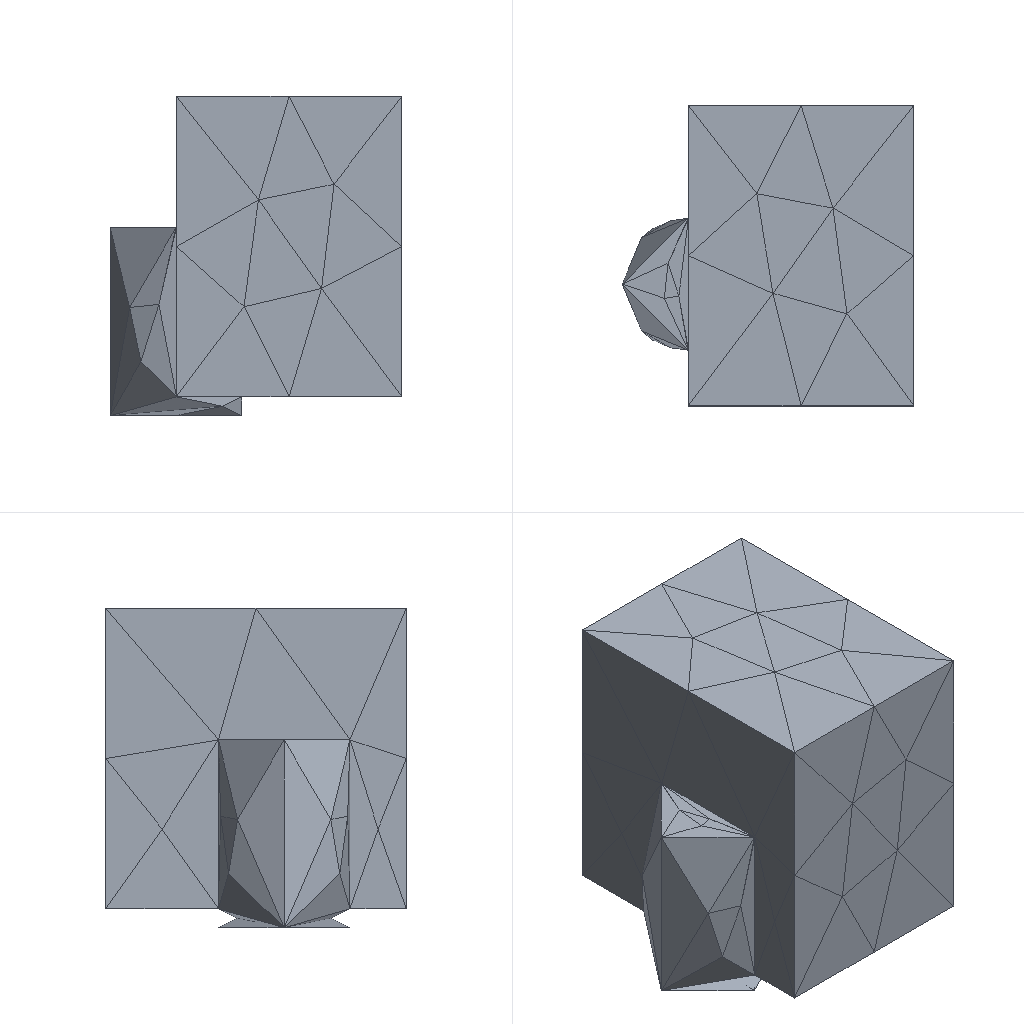Simulation study | ansys mapdl
Set-up summary:
category,name,step,type,value,unit,region
solver,ansys_mapdl
units,mm-N-s-tonne (MPa),,inferred,E=210000 density=
analysis,model,,static
mesh,nodes,,,381
mesh,elements,,,178
element_type,SOLID187,,,178
material,mat 1,,E,210000
material,mat 1,,nu,0.3
load,,model,body load temp,,,all
load,,model,force,"1000 [dir=(0, 0, -1) n=73]",,node list
bc,,model,fixed,"[dofs=UX,UY,UZ n=528]",,node list
Ansys APDL input file, long lists of numbers shortened:
/COM,ANSYS RELEASE 2026 R1           BUILD 26.1      UP20260202       09:11:09
/PREP7
/NOPR
/TITLE,2
ANTYPE, 0
*IF,_CDRDOFF,EQ,1,THEN     !if solid model was read in
_CDRDOFF=             !reset flag, numoffs already performed
*ELSE              !offset database for the following FE model
NUMOFF,NODE,      381
NUMOFF,ELEM,      178
NUMOFF,MAT ,        1
NUMOFF,TYPE,        1
*ENDIF
*SET,_RETURN ,  0.
*SET,_STATUS ,  0.
*SET,_UIQR   ,  73.
*SET,__FLOATPARAMETER__,  381.
DOF,DELETE
ETBLOCK,        1,        1
(2i9,19a9)
        1      187        0        0        0        0        0        0        0        0        0        0        0        0        0        0        0        0        0        0        0
       -1
NBLOCK,6,SOLID,       381,       381
(3i9,6e21.13e3)
        1        0        0 3.9473805561821E+001-1.5006783582075E+000-1.0000000000000E+000
! (380 more lines like these left out)
N,UNBL,LOC,       -1,
EBLOCK,19,SOLID,       178,       178
(19i10)
         1         1         1         1         0         0         0         0        10         0         1       251       252       253        83       258       259       260       261
! (355 more lines like these left out)
        -1
MPTEMP,UNBL, 1, 1,  0.    ,
MPDATA,UNBL, 1,EX  ,       1, 1,  210000.000    ,
MPTEMP,UNBL, 1, 1,  0.    ,
MPDATA,UNBL, 1,NUXY,       1, 1, 0.3    ,
MPTEMP,UNBL, 1, 1,  0.    ,
MPDATA,UNBL, 1,PRXY,       1, 1, 0.3    ,
EXTOPT,ATTR,      0,      0,      0
EXTOPT,ESIZE,  0,  0.
EXTOPT,ACLEAR,      0
TREF,  0.
IRLF,  0
BFUNIF,TEMP,_TINY
ACEL,  0.    ,  0.    ,  0.
OMEGA,  0.    ,  0.    ,  0.
DOMEGA,  0.    ,  0.    ,  0.
CGLOC,  0.    ,  0.    ,  0.
CGOMEGA,  0.    ,  0.    ,  0.
DCGOMG,  0.    ,  0.    ,  0.
KUSE,     0
TIME,  0.
ALPHAD,  0.
BETAD,  0.
DMPRAT,  0.
DMPSTR,  0.
CRPLIM, 0.1    ,   0
CRPLIM,  0.    ,   1
NCNV,     0, 1.000000000E+12,     0,  0.    ,  0.
NEQIT,     0
ERESX,DEFA
DBLOCK,       528
(i9,a6,2(pg16.9))
        1  UX    0.00000000      0.00000000
! (527 more lines like these left out)
       -1
FBLOCK,        73
(i9,a6,2(pg16.9))
       90  FZ   -13.6986301      0.00000000
! (72 more lines like these left out)
       -1
/GO
FINISH
Results summary:
result,analysis_type_db,,,static,unstated
result,n_sets,,,1,unstated
result,load_steps[0].set,load_step=1,,1,unstated
result,load_steps[0].substep,load_step=1,,1,unstated
result,load_steps[0].time,load_step=1,,1,unstated
result,load_steps[0].freq,load_step=1,,1,unstated
result,load_steps[0].max_usum,load_step=1,,0.0004691,unstated
result,load_steps[0].max_seqv,load_step=1,,9.497,unstated
result,load_steps[0].reaction_sum.FX,load_step=1,,-2.78316e-12,unstated
result,load_steps[0].reaction_sum.FY,load_step=1,,3.1543e-11,unstated
result,load_steps[0].reaction_sum.FZ,load_step=1,,1000,unstated
result,load_steps[0].reaction_sum.MX,load_step=1,,0,unstated
result,load_steps[0].reaction_sum.MY,load_step=1,,0,unstated
result,load_steps[0].reaction_sum.MZ,load_step=1,,0,unstated
result,convergence,,,results present for all listed sets,unstated